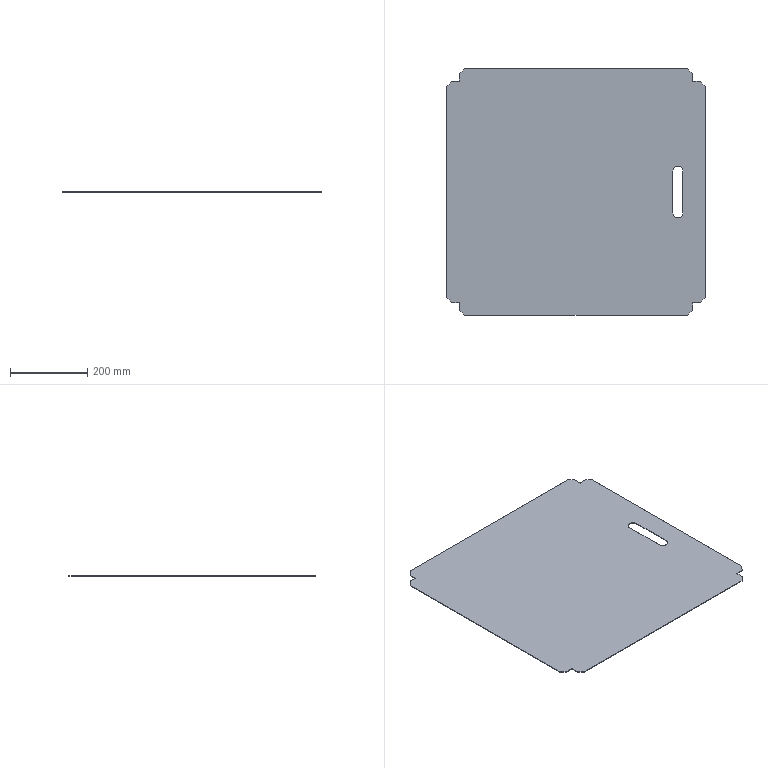Part | SolidWorks | features EdgeFlange 2, FlatPattern 1, ICE 1, SMBaseFlange 1, SheetMetal 1 | 1 solid | 42 faces | box 668.448 x 638.448 x 1.5 mm | volume 627538 mm3 | plane 40 | cylinder 2 | commonest cylinder face diameters 26 x2
STEP:
#1=CARTESIAN_POINT('',(276.5,54.,-1.5));
#2=VERTEX_POINT('',#1);
#3=CARTESIAN_POINT('',(276.5,-54.,-1.5));
#4=VERTEX_POINT('',#3);
#5=CARTESIAN_POINT('',(276.5,54.,-1.5));
#6=DIRECTION('',(0.,-1.,0.));
#7=VECTOR('',#6,1000.);
#8=LINE('',#5,#7);
#9=EDGE_CURVE('',#2,#4,#8,.T.);
#10=ORIENTED_EDGE('',*,*,#9,.F.);
#11=CARTESIAN_POINT('',(250.5,54.,-1.5));
#12=VERTEX_POINT('',#11);
#13=CARTESIAN_POINT('',(263.5,54.,-1.5));
#14=DIRECTION('',(0.,0.,-1.));
#15=DIRECTION('',(-1.,0.,0.));
#16=AXIS2_PLACEMENT_3D('',#13,#14,#15);
#17=CIRCLE('',#16,13.);
#18=EDGE_CURVE('',#12,#2,#17,.T.);
#19=ORIENTED_EDGE('',*,*,#18,.F.);
#20=CARTESIAN_POINT('',(250.5,-54.,-1.5));
#21=VERTEX_POINT('',#20);
#22=CARTESIAN_POINT('',(250.5,54.,-1.5));
#23=DIRECTION('',(0.,1.,0.));
#24=VECTOR('',#23,1000.);
#25=LINE('',#22,#24);
#26=EDGE_CURVE('',#21,#12,#25,.T.);
#27=ORIENTED_EDGE('',*,*,#26,.F.);
#28=CARTESIAN_POINT('',(263.5,-54.,-1.5));
#29=DIRECTION('',(0.,0.,-1.));
#30=DIRECTION('',(-1.,0.,0.));
#31=AXIS2_PLACEMENT_3D('',#28,#29,#30);
#32=CIRCLE('',#31,13.);
#33=EDGE_CURVE('',#4,#21,#32,.T.);
#34=ORIENTED_EDGE('',*,*,#33,.F.);
#35=EDGE_LOOP('',(#10,#19,#27,#34));
#36=FACE_BOUND('',#35,.T.);
#37=CARTESIAN_POINT('',(303.599,-286.293,-1.5));
#38=VERTEX_POINT('',#37);
#39=CARTESIAN_POINT('',(301.263,-286.263,-1.5));
#40=VERTEX_POINT('',#39);
#41=CARTESIAN_POINT('',(303.599,-286.293,-1.5));
#42=DIRECTION('',(-0.9999,0.01263,0.));
#43=VECTOR('',#42,1000.);
#44=LINE('',#41,#43);
#45=EDGE_CURVE('',#38,#40,#44,.T.);
#46=ORIENTED_EDGE('',*,*,#45,.T.);
#47=CARTESIAN_POINT('',(301.293,-286.293,-1.5));
#48=VERTEX_POINT('',#47);
#49=CARTESIAN_POINT('',(301.278,-286.278,-1.5));
#50=DIRECTION('',(-0.7071,0.7071,0.));
#51=VECTOR('',#50,1000.);
#52=LINE('',#49,#51);
#53=EDGE_CURVE('',#48,#40,#52,.T.);
#54=ORIENTED_EDGE('',*,*,#53,.F.);
#55=CARTESIAN_POINT('',(301.293,-304.125,-1.5));
#56=VERTEX_POINT('',#55);
#57=CARTESIAN_POINT('',(301.293,-287.862,-1.5));
#58=DIRECTION('',(0.,-1.,0.));
#59=VECTOR('',#58,1000.);
#60=LINE('',#57,#59);
#61=EDGE_CURVE('',#48,#56,#60,.T.);
#62=ORIENTED_EDGE('',*,*,#61,.T.);
#63=CARTESIAN_POINT('',(300.556,-306.46,-1.5));
#64=VERTEX_POINT('',#63);
#65=CARTESIAN_POINT('',(301.293,-304.125,-1.5));
#66=DIRECTION('',(-0.3008,-0.9537,0.));
#67=VECTOR('',#66,1000.);
#68=LINE('',#65,#67);
#69=EDGE_CURVE('',#56,#64,#68,.T.);
#70=ORIENTED_EDGE('',*,*,#69,.T.);
#71=CARTESIAN_POINT('',(287.793,-319.224,-1.5));
#72=VERTEX_POINT('',#71);
#73=CARTESIAN_POINT('',(-124.592,-731.608,-1.5));
#74=DIRECTION('',(0.7071,0.7071,0.));
#75=VECTOR('',#74,1000.);
#76=LINE('',#73,#75);
#77=EDGE_CURVE('',#72,#64,#76,.T.);
#78=ORIENTED_EDGE('',*,*,#77,.F.);
#79=CARTESIAN_POINT('',(-287.793,-319.224,-1.5));
#80=VERTEX_POINT('',#79);
#81=CARTESIAN_POINT('',(0.,-319.224,-1.5));
#82=DIRECTION('',(-1.,0.,0.));
#83=VECTOR('',#82,1000.);
#84=LINE('',#81,#83);
#85=EDGE_CURVE('',#72,#80,#84,.T.);
#86=ORIENTED_EDGE('',*,*,#85,.T.);
#87=CARTESIAN_POINT('',(-300.556,-306.46,-1.5));
#88=VERTEX_POINT('',#87);
#89=CARTESIAN_POINT('',(-300.556,-306.46,-1.5));
#90=DIRECTION('',(0.7071,-0.7071,0.));
#91=VECTOR('',#90,1000.);
#92=LINE('',#89,#91);
#93=EDGE_CURVE('',#88,#80,#92,.T.);
#94=ORIENTED_EDGE('',*,*,#93,.F.);
#95=CARTESIAN_POINT('',(-301.293,-304.125,-1.5));
#96=VERTEX_POINT('',#95);
#97=CARTESIAN_POINT('',(-300.556,-306.46,-1.5));
#98=DIRECTION('',(-0.3008,0.9537,0.));
#99=VECTOR('',#98,1000.);
#100=LINE('',#97,#99);
#101=EDGE_CURVE('',#88,#96,#100,.T.);
#102=ORIENTED_EDGE('',*,*,#101,.T.);
#103=CARTESIAN_POINT('',(-301.293,-288.599,-1.5));
#104=VERTEX_POINT('',#103);
#105=CARTESIAN_POINT('',(-301.293,-287.862,-1.5));
#106=DIRECTION('',(0.,-1.,0.));
#107=VECTOR('',#106,1000.);
#108=LINE('',#105,#107);
#109=EDGE_CURVE('',#104,#96,#108,.T.);
#110=ORIENTED_EDGE('',*,*,#109,.F.);
#111=CARTESIAN_POINT('',(-301.263,-286.263,-1.5));
#112=VERTEX_POINT('',#111);
#113=CARTESIAN_POINT('',(-301.293,-288.599,-1.5));
#114=DIRECTION('',(0.01263,0.9999,0.));
#115=VECTOR('',#114,1000.);
#116=LINE('',#113,#115);
#117=EDGE_CURVE('',#104,#112,#116,.T.);
#118=ORIENTED_EDGE('',*,*,#117,.T.);
#119=CARTESIAN_POINT('',(-301.293,-286.293,-1.5));
#120=VERTEX_POINT('',#119);
#121=CARTESIAN_POINT('',(-301.278,-286.278,-1.5));
#122=DIRECTION('',(0.7071,0.7071,0.));
#123=VECTOR('',#122,1000.);
#124=LINE('',#121,#123);
#125=EDGE_CURVE('',#120,#112,#124,.T.);
#126=ORIENTED_EDGE('',*,*,#125,.F.);
#127=CARTESIAN_POINT('',(-319.125,-286.293,-1.5));
#128=VERTEX_POINT('',#127);
#129=CARTESIAN_POINT('',(-302.862,-286.293,-1.5));
#130=DIRECTION('',(-1.,0.,0.));
#131=VECTOR('',#130,1000.);
#132=LINE('',#129,#131);
#133=EDGE_CURVE('',#120,#128,#132,.T.);
#134=ORIENTED_EDGE('',*,*,#133,.T.);
#135=CARTESIAN_POINT('',(-321.46,-285.556,-1.5));
#136=VERTEX_POINT('',#135);
#137=CARTESIAN_POINT('',(-319.125,-286.293,-1.5));
#138=DIRECTION('',(-0.9537,0.3008,0.));
#139=VECTOR('',#138,1000.);
#140=LINE('',#137,#139);
#141=EDGE_CURVE('',#128,#136,#140,.T.);
#142=ORIENTED_EDGE('',*,*,#141,.T.);
#143=CARTESIAN_POINT('',(-334.224,-272.793,-1.5));
#144=VERTEX_POINT('',#143);
#145=CARTESIAN_POINT('',(-725.4,118.384,-1.5));
#146=DIRECTION('',(0.7071,-0.7071,0.));
#147=VECTOR('',#146,1000.);
#148=LINE('',#145,#147);
#149=EDGE_CURVE('',#144,#136,#148,.T.);
#150=ORIENTED_EDGE('',*,*,#149,.F.);
#151=CARTESIAN_POINT('',(-334.224,272.793,-1.5));
#152=VERTEX_POINT('',#151);
#153=CARTESIAN_POINT('',(-334.224,0.,-1.5));
#154=DIRECTION('',(0.,1.,0.));
#155=VECTOR('',#154,1000.);
#156=LINE('',#153,#155);
#157=EDGE_CURVE('',#144,#152,#156,.T.);
#158=ORIENTED_EDGE('',*,*,#157,.T.);
#159=CARTESIAN_POINT('',(-321.46,285.556,-1.5));
#160=VERTEX_POINT('',#159);
#161=CARTESIAN_POINT('',(-321.46,285.556,-1.5));
#162=DIRECTION('',(-0.7071,-0.7071,0.));
#163=VECTOR('',#162,1000.);
#164=LINE('',#161,#163);
#165=EDGE_CURVE('',#160,#152,#164,.T.);
#166=ORIENTED_EDGE('',*,*,#165,.F.);
#167=CARTESIAN_POINT('',(-319.125,286.293,-1.5));
#168=VERTEX_POINT('',#167);
#169=CARTESIAN_POINT('',(-321.46,285.556,-1.5));
#170=DIRECTION('',(0.9537,0.3008,0.));
#171=VECTOR('',#170,1000.);
#172=LINE('',#169,#171);
#173=EDGE_CURVE('',#160,#168,#172,.T.);
#174=ORIENTED_EDGE('',*,*,#173,.T.);
#175=CARTESIAN_POINT('',(-303.599,286.293,-1.5));
#176=VERTEX_POINT('',#175);
#177=CARTESIAN_POINT('',(-302.862,286.293,-1.5));
#178=DIRECTION('',(-1.,0.,0.));
#179=VECTOR('',#178,1000.);
#180=LINE('',#177,#179);
#181=EDGE_CURVE('',#176,#168,#180,.T.);
#182=ORIENTED_EDGE('',*,*,#181,.F.);
#183=CARTESIAN_POINT('',(-301.263,286.263,-1.5));
#184=VERTEX_POINT('',#183);
#185=CARTESIAN_POINT('',(-303.599,286.293,-1.5));
#186=DIRECTION('',(0.9999,-0.01263,0.));
#187=VECTOR('',#186,1000.);
#188=LINE('',#185,#187);
#189=EDGE_CURVE('',#176,#184,#188,.T.);
#190=ORIENTED_EDGE('',*,*,#189,.T.);
#191=CARTESIAN_POINT('',(-301.293,286.293,-1.5));
#192=VERTEX_POINT('',#191);
#193=CARTESIAN_POINT('',(-301.278,286.278,-1.5));
#194=DIRECTION('',(0.7071,-0.7071,0.));
#195=VECTOR('',#194,1000.);
#196=LINE('',#193,#195);
#197=EDGE_CURVE('',#192,#184,#196,.T.);
#198=ORIENTED_EDGE('',*,*,#197,.F.);
#199=CARTESIAN_POINT('',(-301.293,304.125,-1.5));
#200=VERTEX_POINT('',#199);
#201=CARTESIAN_POINT('',(-301.293,287.862,-1.5));
#202=DIRECTION('',(0.,1.,0.));
#203=VECTOR('',#202,1000.);
#204=LINE('',#201,#203);
#205=EDGE_CURVE('',#192,#200,#204,.T.);
#206=ORIENTED_EDGE('',*,*,#205,.T.);
#207=CARTESIAN_POINT('',(-300.556,306.46,-1.5));
#208=VERTEX_POINT('',#207);
#209=CARTESIAN_POINT('',(-301.293,304.125,-1.5));
#210=DIRECTION('',(0.3008,0.9537,0.));
#211=VECTOR('',#210,1000.);
#212=LINE('',#209,#211);
#213=EDGE_CURVE('',#200,#208,#212,.T.);
#214=ORIENTED_EDGE('',*,*,#213,.T.);
#215=CARTESIAN_POINT('',(-287.793,319.224,-1.5));
#216=VERTEX_POINT('',#215);
#217=CARTESIAN_POINT('',(124.592,731.608,-1.5));
#218=DIRECTION('',(-0.7071,-0.7071,0.));
#219=VECTOR('',#218,1000.);
#220=LINE('',#217,#219);
#221=EDGE_CURVE('',#216,#208,#220,.T.);
#222=ORIENTED_EDGE('',*,*,#221,.F.);
#223=CARTESIAN_POINT('',(287.793,319.224,-1.5));
#224=VERTEX_POINT('',#223);
#225=CARTESIAN_POINT('',(0.,319.224,-1.5));
#226=DIRECTION('',(1.,0.,0.));
#227=VECTOR('',#226,1000.);
#228=LINE('',#225,#227);
#229=EDGE_CURVE('',#216,#224,#228,.T.);
#230=ORIENTED_EDGE('',*,*,#229,.T.);
#231=CARTESIAN_POINT('',(300.556,306.46,-1.5));
#232=VERTEX_POINT('',#231);
#233=CARTESIAN_POINT('',(300.556,306.46,-1.5));
#234=DIRECTION('',(-0.7071,0.7071,0.));
#235=VECTOR('',#234,1000.);
#236=LINE('',#233,#235);
#237=EDGE_CURVE('',#232,#224,#236,.T.);
#238=ORIENTED_EDGE('',*,*,#237,.F.);
#239=CARTESIAN_POINT('',(301.293,304.125,-1.5));
#240=VERTEX_POINT('',#239);
#241=CARTESIAN_POINT('',(300.556,306.46,-1.5));
#242=DIRECTION('',(0.3008,-0.9537,0.));
#243=VECTOR('',#242,1000.);
#244=LINE('',#241,#243);
#245=EDGE_CURVE('',#232,#240,#244,.T.);
#246=ORIENTED_EDGE('',*,*,#245,.T.);
#247=CARTESIAN_POINT('',(301.293,288.599,-1.5));
#248=VERTEX_POINT('',#247);
#249=CARTESIAN_POINT('',(301.293,287.862,-1.5));
#250=DIRECTION('',(0.,1.,0.));
#251=VECTOR('',#250,1000.);
#252=LINE('',#249,#251);
#253=EDGE_CURVE('',#248,#240,#252,.T.);
#254=ORIENTED_EDGE('',*,*,#253,.F.);
#255=CARTESIAN_POINT('',(301.263,286.263,-1.5));
#256=VERTEX_POINT('',#255);
#257=CARTESIAN_POINT('',(301.293,288.599,-1.5));
#258=DIRECTION('',(-0.01263,-0.9999,0.));
#259=VECTOR('',#258,1000.);
#260=LINE('',#257,#259);
#261=EDGE_CURVE('',#248,#256,#260,.T.);
#262=ORIENTED_EDGE('',*,*,#261,.T.);
#263=CARTESIAN_POINT('',(301.293,286.293,-1.5));
#264=VERTEX_POINT('',#263);
#265=CARTESIAN_POINT('',(301.278,286.278,-1.5));
#266=DIRECTION('',(-0.7071,-0.7071,0.));
#267=VECTOR('',#266,1000.);
#268=LINE('',#265,#267);
#269=EDGE_CURVE('',#264,#256,#268,.T.);
#270=ORIENTED_EDGE('',*,*,#269,.F.);
#271=CARTESIAN_POINT('',(319.125,286.293,-1.5));
#272=VERTEX_POINT('',#271);
#273=CARTESIAN_POINT('',(302.862,286.293,-1.5));
#274=DIRECTION('',(1.,0.,0.));
#275=VECTOR('',#274,1000.);
#276=LINE('',#273,#275);
#277=EDGE_CURVE('',#264,#272,#276,.T.);
#278=ORIENTED_EDGE('',*,*,#277,.T.);
#279=CARTESIAN_POINT('',(321.46,285.556,-1.5));
#280=VERTEX_POINT('',#279);
#281=CARTESIAN_POINT('',(319.125,286.293,-1.5));
#282=DIRECTION('',(0.9537,-0.3008,0.));
#283=VECTOR('',#282,1000.);
#284=LINE('',#281,#283);
#285=EDGE_CURVE('',#272,#280,#284,.T.);
#286=ORIENTED_EDGE('',*,*,#285,.T.);
#287=CARTESIAN_POINT('',(334.224,272.793,-1.5));
#288=VERTEX_POINT('',#287);
#289=CARTESIAN_POINT('',(725.4,-118.384,-1.5));
#290=DIRECTION('',(-0.7071,0.7071,0.));
#291=VECTOR('',#290,1000.);
#292=LINE('',#289,#291);
#293=EDGE_CURVE('',#288,#280,#292,.T.);
#294=ORIENTED_EDGE('',*,*,#293,.F.);
#295=CARTESIAN_POINT('',(334.224,-272.793,-1.5));
#296=VERTEX_POINT('',#295);
#297=CARTESIAN_POINT('',(334.224,0.,-1.5));
#298=DIRECTION('',(0.,-1.,0.));
#299=VECTOR('',#298,1000.);
#300=LINE('',#297,#299);
#301=EDGE_CURVE('',#288,#296,#300,.T.);
#302=ORIENTED_EDGE('',*,*,#301,.T.);
#303=CARTESIAN_POINT('',(321.46,-285.556,-1.5));
#304=VERTEX_POINT('',#303);
#305=CARTESIAN_POINT('',(321.46,-285.556,-1.5));
#306=DIRECTION('',(0.7071,0.7071,0.));
#307=VECTOR('',#306,1000.);
#308=LINE('',#305,#307);
#309=EDGE_CURVE('',#304,#296,#308,.T.);
#310=ORIENTED_EDGE('',*,*,#309,.F.);
#311=CARTESIAN_POINT('',(319.125,-286.293,-1.5));
#312=VERTEX_POINT('',#311);
#313=CARTESIAN_POINT('',(321.46,-285.556,-1.5));
#314=DIRECTION('',(-0.9537,-0.3008,0.));
#315=VECTOR('',#314,1000.);
#316=LINE('',#313,#315);
#317=EDGE_CURVE('',#304,#312,#316,.T.);
#318=ORIENTED_EDGE('',*,*,#317,.T.);
#319=CARTESIAN_POINT('',(302.862,-286.293,-1.5));
#320=DIRECTION('',(1.,0.,0.));
#321=VECTOR('',#320,1000.);
#322=LINE('',#319,#321);
#323=EDGE_CURVE('',#38,#312,#322,.T.);
#324=ORIENTED_EDGE('',*,*,#323,.F.);
#325=EDGE_LOOP('',(#46,#54,#62,#70,#78,#86,#94,#102,#110,#118,#126,#134,#142,#150,#158,#166,#174,#182,#190,#198,#206,#214,#222,#230,#238,#246,#254,#262,#270,#278,#286,#294,#302,#310,#318,#324));
#326=FACE_OUTER_BOUND('',#325,.T.);
#327=CARTESIAN_POINT('',(0.,0.,-1.5));
#328=DIRECTION('',(0.,0.,1.));
#329=DIRECTION('',(1.,0.,0.));
#330=AXIS2_PLACEMENT_3D('',#327,#328,#329);
#331=PLANE('',#330);
#332=ADVANCED_FACE('',(#36,#326),#331,.F.);
#333=CARTESIAN_POINT('',(276.5,54.,0.));
#334=VERTEX_POINT('',#333);
#335=CARTESIAN_POINT('',(250.5,54.,0.));
#336=VERTEX_POINT('',#335);
#337=CARTESIAN_POINT('',(263.5,54.,0.));
#338=DIRECTION('',(0.,0.,1.));
#339=DIRECTION('',(1.,0.,0.));
#340=AXIS2_PLACEMENT_3D('',#337,#338,#339);
#341=CIRCLE('',#340,13.);
#342=EDGE_CURVE('',#334,#336,#341,.T.);
#343=ORIENTED_EDGE('',*,*,#342,.F.);
#344=CARTESIAN_POINT('',(276.5,-54.,0.));
#345=VERTEX_POINT('',#344);
#346=CARTESIAN_POINT('',(276.5,0.,0.));
#347=DIRECTION('',(0.,1.,0.));
#348=VECTOR('',#347,1000.);
#349=LINE('',#346,#348);
#350=EDGE_CURVE('',#345,#334,#349,.T.);
#351=ORIENTED_EDGE('',*,*,#350,.F.);
#352=CARTESIAN_POINT('',(250.5,-54.,0.));
#353=VERTEX_POINT('',#352);
#354=CARTESIAN_POINT('',(263.5,-54.,0.));
#355=DIRECTION('',(0.,0.,1.));
#356=DIRECTION('',(1.,0.,0.));
#357=AXIS2_PLACEMENT_3D('',#354,#355,#356);
#358=CIRCLE('',#357,13.);
#359=EDGE_CURVE('',#353,#345,#358,.T.);
#360=ORIENTED_EDGE('',*,*,#359,.F.);
#361=CARTESIAN_POINT('',(250.5,0.,0.));
#362=DIRECTION('',(0.,-1.,0.));
#363=VECTOR('',#362,1000.);
#364=LINE('',#361,#363);
#365=EDGE_CURVE('',#336,#353,#364,.T.);
#366=ORIENTED_EDGE('',*,*,#365,.F.);
#367=EDGE_LOOP('',(#343,#351,#360,#366));
#368=FACE_BOUND('',#367,.T.);
#369=CARTESIAN_POINT('',(-301.293,-286.293,0.));
#370=VERTEX_POINT('',#369);
#371=CARTESIAN_POINT('',(-301.263,-286.263,0.));
#372=VERTEX_POINT('',#371);
#373=CARTESIAN_POINT('',(-301.278,-286.278,0.));
#374=DIRECTION('',(0.7071,0.7071,0.));
#375=VECTOR('',#374,1000.);
#376=LINE('',#373,#375);
#377=EDGE_CURVE('',#370,#372,#376,.T.);
#378=ORIENTED_EDGE('',*,*,#377,.T.);
#379=CARTESIAN_POINT('',(-301.293,-288.599,0.));
#380=VERTEX_POINT('',#379);
#381=CARTESIAN_POINT('',(-301.293,-288.599,0.));
#382=DIRECTION('',(0.01263,0.9999,0.));
#383=VECTOR('',#382,1000.);
#384=LINE('',#381,#383);
#385=EDGE_CURVE('',#380,#372,#384,.T.);
#386=ORIENTED_EDGE('',*,*,#385,.F.);
#387=CARTESIAN_POINT('',(-301.293,-304.125,0.));
#388=VERTEX_POINT('',#387);
#389=CARTESIAN_POINT('',(-301.293,-287.862,0.));
#390=DIRECTION('',(0.,-1.,0.));
#391=VECTOR('',#390,1000.);
#392=LINE('',#389,#391);
#393=EDGE_CURVE('',#380,#388,#392,.T.);
#394=ORIENTED_EDGE('',*,*,#393,.T.);
#395=CARTESIAN_POINT('',(-300.556,-306.46,0.));
#396=VERTEX_POINT('',#395);
#397=CARTESIAN_POINT('',(-300.556,-306.46,0.));
#398=DIRECTION('',(-0.3008,0.9537,0.));
#399=VECTOR('',#398,1000.);
#400=LINE('',#397,#399);
#401=EDGE_CURVE('',#396,#388,#400,.T.);
#402=ORIENTED_EDGE('',*,*,#401,.F.);
#403=CARTESIAN_POINT('',(-287.793,-319.224,0.));
#404=VERTEX_POINT('',#403);
#405=CARTESIAN_POINT('',(-7.146,-599.87,0.));
#406=DIRECTION('',(0.7071,-0.7071,0.));
#407=VECTOR('',#406,1000.);
#408=LINE('',#405,#407);
#409=EDGE_CURVE('',#396,#404,#408,.T.);
#410=ORIENTED_EDGE('',*,*,#409,.T.);
#411=CARTESIAN_POINT('',(287.793,-319.224,0.));
#412=VERTEX_POINT('',#411);
#413=CARTESIAN_POINT('',(-301.293,-319.224,0.));
#414=DIRECTION('',(-1.,0.,0.));
#415=VECTOR('',#414,1000.);
#416=LINE('',#413,#415);
#417=EDGE_CURVE('',#412,#404,#416,.T.);
#418=ORIENTED_EDGE('',*,*,#417,.F.);
#419=CARTESIAN_POINT('',(300.556,-306.46,0.));
#420=VERTEX_POINT('',#419);
#421=CARTESIAN_POINT('',(7.146,-599.87,0.));
#422=DIRECTION('',(0.7071,0.7071,0.));
#423=VECTOR('',#422,1000.);
#424=LINE('',#421,#423);
#425=EDGE_CURVE('',#412,#420,#424,.T.);
#426=ORIENTED_EDGE('',*,*,#425,.T.);
#427=CARTESIAN_POINT('',(301.293,-304.125,0.));
#428=VERTEX_POINT('',#427);
#429=CARTESIAN_POINT('',(301.293,-304.125,0.));
#430=DIRECTION('',(-0.3008,-0.9537,0.));
#431=VECTOR('',#430,1000.);
#432=LINE('',#429,#431);
#433=EDGE_CURVE('',#428,#420,#432,.T.);
#434=ORIENTED_EDGE('',*,*,#433,.F.);
#435=CARTESIAN_POINT('',(301.293,-286.293,0.));
#436=VERTEX_POINT('',#435);
#437=CARTESIAN_POINT('',(301.293,-287.862,0.));
#438=DIRECTION('',(0.,-1.,0.));
#439=VECTOR('',#438,1000.);
#440=LINE('',#437,#439);
#441=EDGE_CURVE('',#436,#428,#440,.T.);
#442=ORIENTED_EDGE('',*,*,#441,.F.);
#443=CARTESIAN_POINT('',(301.263,-286.263,0.));
#444=VERTEX_POINT('',#443);
#445=CARTESIAN_POINT('',(301.278,-286.278,0.));
#446=DIRECTION('',(-0.7071,0.7071,0.));
#447=VECTOR('',#446,1000.);
#448=LINE('',#445,#447);
#449=EDGE_CURVE('',#436,#444,#448,.T.);
#450=ORIENTED_EDGE('',*,*,#449,.T.);
#451=CARTESIAN_POINT('',(303.599,-286.293,0.));
#452=VERTEX_POINT('',#451);
#453=CARTESIAN_POINT('',(303.599,-286.293,0.));
#454=DIRECTION('',(-0.9999,0.01263,0.));
#455=VECTOR('',#454,1000.);
#456=LINE('',#453,#455);
#457=EDGE_CURVE('',#452,#444,#456,.T.);
#458=ORIENTED_EDGE('',*,*,#457,.F.);
#459=CARTESIAN_POINT('',(319.125,-286.293,0.));
#460=VERTEX_POINT('',#459);
#461=CARTESIAN_POINT('',(302.862,-286.293,0.));
#462=DIRECTION('',(1.,0.,0.));
#463=VECTOR('',#462,1000.);
#464=LINE('',#461,#463);
#465=EDGE_CURVE('',#452,#460,#464,.T.);
#466=ORIENTED_EDGE('',*,*,#465,.T.);
#467=CARTESIAN_POINT('',(321.46,-285.556,0.));
#468=VERTEX_POINT('',#467);
#469=CARTESIAN_POINT('',(321.46,-285.556,0.));
#470=DIRECTION('',(-0.9537,-0.3008,0.));
#471=VECTOR('',#470,1000.);
#472=LINE('',#469,#471);
#473=EDGE_CURVE('',#468,#460,#472,.T.);
#474=ORIENTED_EDGE('',*,*,#473,.F.);
#475=CARTESIAN_POINT('',(334.224,-272.793,0.));
#476=VERTEX_POINT('',#475);
#477=CARTESIAN_POINT('',(614.87,7.854,0.));
#478=DIRECTION('',(0.7071,0.7071,0.));
#479=VECTOR('',#478,1000.);
#480=LINE('',#477,#479);
#481=EDGE_CURVE('',#468,#476,#480,.T.);
#482=ORIENTED_EDGE('',*,*,#481,.T.);
#483=CARTESIAN_POINT('',(334.224,272.793,0.));
#484=VERTEX_POINT('',#483);
#485=CARTESIAN_POINT('',(334.224,-286.293,0.));
#486=DIRECTION('',(0.,-1.,0.));
#487=VECTOR('',#486,1000.);
#488=LINE('',#485,#487);
#489=EDGE_CURVE('',#484,#476,#488,.T.);
#490=ORIENTED_EDGE('',*,*,#489,.F.);
#491=CARTESIAN_POINT('',(321.46,285.556,0.));
#492=VERTEX_POINT('',#491);
#493=CARTESIAN_POINT('',(614.87,-7.854,0.));
#494=DIRECTION('',(-0.7071,0.7071,0.));
#495=VECTOR('',#494,1000.);
#496=LINE('',#493,#495);
#497=EDGE_CURVE('',#484,#492,#496,.T.);
#498=ORIENTED_EDGE('',*,*,#497,.T.);
#499=CARTESIAN_POINT('',(319.125,286.293,0.));
#500=VERTEX_POINT('',#499);
#501=CARTESIAN_POINT('',(319.125,286.293,0.));
#502=DIRECTION('',(0.9537,-0.3008,0.));
#503=VECTOR('',#502,1000.);
#504=LINE('',#501,#503);
#505=EDGE_CURVE('',#500,#492,#504,.T.);
#506=ORIENTED_EDGE('',*,*,#505,.F.);
#507=CARTESIAN_POINT('',(301.293,286.293,0.));
#508=VERTEX_POINT('',#507);
#509=CARTESIAN_POINT('',(302.862,286.293,0.));
#510=DIRECTION('',(1.,0.,0.));
#511=VECTOR('',#510,1000.);
#512=LINE('',#509,#511);
#513=EDGE_CURVE('',#508,#500,#512,.T.);
#514=ORIENTED_EDGE('',*,*,#513,.F.);
#515=CARTESIAN_POINT('',(301.263,286.263,0.));
#516=VERTEX_POINT('',#515);
#517=CARTESIAN_POINT('',(301.278,286.278,0.));
#518=DIRECTION('',(-0.7071,-0.7071,0.));
#519=VECTOR('',#518,1000.);
#520=LINE('',#517,#519);
#521=EDGE_CURVE('',#508,#516,#520,.T.);
#522=ORIENTED_EDGE('',*,*,#521,.T.);
#523=CARTESIAN_POINT('',(301.293,288.599,0.));
#524=VERTEX_POINT('',#523);
#525=CARTESIAN_POINT('',(301.293,288.599,0.));
#526=DIRECTION('',(-0.01263,-0.9999,0.));
#527=VECTOR('',#526,1000.);
#528=LINE('',#525,#527);
#529=EDGE_CURVE('',#524,#516,#528,.T.);
#530=ORIENTED_EDGE('',*,*,#529,.F.);
#531=CARTESIAN_POINT('',(301.293,304.125,0.));
#532=VERTEX_POINT('',#531);
#533=CARTESIAN_POINT('',(301.293,287.862,0.));
#534=DIRECTION('',(0.,1.,0.));
#535=VECTOR('',#534,1000.);
#536=LINE('',#533,#535);
#537=EDGE_CURVE('',#524,#532,#536,.T.);
#538=ORIENTED_EDGE('',*,*,#537,.T.);
#539=CARTESIAN_POINT('',(300.556,306.46,0.));
#540=VERTEX_POINT('',#539);
#541=CARTESIAN_POINT('',(300.556,306.46,0.));
#542=DIRECTION('',(0.3008,-0.9537,0.));
#543=VECTOR('',#542,1000.);
#544=LINE('',#541,#543);
#545=EDGE_CURVE('',#540,#532,#544,.T.);
#546=ORIENTED_EDGE('',*,*,#545,.F.);
#547=CARTESIAN_POINT('',(287.793,319.224,0.));
#548=VERTEX_POINT('',#547);
#549=CARTESIAN_POINT('',(7.146,599.87,0.));
#550=DIRECTION('',(-0.7071,0.7071,0.));
#551=VECTOR('',#550,1000.);
#552=LINE('',#549,#551);
#553=EDGE_CURVE('',#540,#548,#552,.T.);
#554=ORIENTED_EDGE('',*,*,#553,.T.);
#555=CARTESIAN_POINT('',(-287.793,319.224,0.));
#556=VERTEX_POINT('',#555);
#557=CARTESIAN_POINT('',(301.293,319.224,0.));
#558=DIRECTION('',(1.,0.,0.));
#559=VECTOR('',#558,1000.);
#560=LINE('',#557,#559);
#561=EDGE_CURVE('',#556,#548,#560,.T.);
#562=ORIENTED_EDGE('',*,*,#561,.F.);
#563=CARTESIAN_POINT('',(-300.556,306.46,0.));
#564=VERTEX_POINT('',#563);
#565=CARTESIAN_POINT('',(-7.146,599.87,0.));
#566=DIRECTION('',(-0.7071,-0.7071,0.));
#567=VECTOR('',#566,1000.);
#568=LINE('',#565,#567);
#569=EDGE_CURVE('',#556,#564,#568,.T.);
#570=ORIENTED_EDGE('',*,*,#569,.T.);
#571=CARTESIAN_POINT('',(-301.293,304.125,0.));
#572=VERTEX_POINT('',#571);
#573=CARTESIAN_POINT('',(-301.293,304.125,0.));
#574=DIRECTION('',(0.3008,0.9537,0.));
#575=VECTOR('',#574,1000.);
#576=LINE('',#573,#575);
#577=EDGE_CURVE('',#572,#564,#576,.T.);
#578=ORIENTED_EDGE('',*,*,#577,.F.);
#579=CARTESIAN_POINT('',(-301.293,286.293,0.));
#580=VERTEX_POINT('',#579);
#581=CARTESIAN_POINT('',(-301.293,287.862,0.));
#582=DIRECTION('',(0.,1.,0.));
#583=VECTOR('',#582,1000.);
#584=LINE('',#581,#583);
#585=EDGE_CURVE('',#580,#572,#584,.T.);
#586=ORIENTED_EDGE('',*,*,#585,.F.);
#587=CARTESIAN_POINT('',(-301.263,286.263,0.));
#588=VERTEX_POINT('',#587);
#589=CARTESIAN_POINT('',(-301.278,286.278,0.));
#590=DIRECTION('',(0.7071,-0.7071,0.));
#591=VECTOR('',#590,1000.);
#592=LINE('',#589,#591);
#593=EDGE_CURVE('',#580,#588,#592,.T.);
#594=ORIENTED_EDGE('',*,*,#593,.T.);
#595=CARTESIAN_POINT('',(-303.599,286.293,0.));
#596=VERTEX_POINT('',#595);
#597=CARTESIAN_POINT('',(-303.599,286.293,0.));
#598=DIRECTION('',(0.9999,-0.01263,0.));
#599=VECTOR('',#598,1000.);
#600=LINE('',#597,#599);
#601=EDGE_CURVE('',#596,#588,#600,.T.);
#602=ORIENTED_EDGE('',*,*,#601,.F.);
#603=CARTESIAN_POINT('',(-319.125,286.293,0.));
#604=VERTEX_POINT('',#603);
#605=CARTESIAN_POINT('',(-302.862,286.293,0.));
#606=DIRECTION('',(-1.,0.,0.));
#607=VECTOR('',#606,1000.);
#608=LINE('',#605,#607);
#609=EDGE_CURVE('',#596,#604,#608,.T.);
#610=ORIENTED_EDGE('',*,*,#609,.T.);
#611=CARTESIAN_POINT('',(-321.46,285.556,0.));
#612=VERTEX_POINT('',#611);
#613=CARTESIAN_POINT('',(-321.46,285.556,0.));
#614=DIRECTION('',(0.9537,0.3008,0.));
#615=VECTOR('',#614,1000.);
#616=LINE('',#613,#615);
#617=EDGE_CURVE('',#612,#604,#616,.T.);
#618=ORIENTED_EDGE('',*,*,#617,.F.);
#619=CARTESIAN_POINT('',(-334.224,272.793,0.));
#620=VERTEX_POINT('',#619);
#621=CARTESIAN_POINT('',(-614.87,-7.854,0.));
#622=DIRECTION('',(-0.7071,-0.7071,0.));
#623=VECTOR('',#622,1000.);
#624=LINE('',#621,#623);
#625=EDGE_CURVE('',#612,#620,#624,.T.);
#626=ORIENTED_EDGE('',*,*,#625,.T.);
#627=CARTESIAN_POINT('',(-334.224,-272.793,0.));
#628=VERTEX_POINT('',#627);
#629=CARTESIAN_POINT('',(-334.224,286.293,0.));
#630=DIRECTION('',(0.,1.,0.));
#631=VECTOR('',#630,1000.);
#632=LINE('',#629,#631);
#633=EDGE_CURVE('',#628,#620,#632,.T.);
#634=ORIENTED_EDGE('',*,*,#633,.F.);
#635=CARTESIAN_POINT('',(-321.46,-285.556,0.));
#636=VERTEX_POINT('',#635);
#637=CARTESIAN_POINT('',(-614.87,7.854,0.));
#638=DIRECTION('',(0.7071,-0.7071,0.));
#639=VECTOR('',#638,1000.);
#640=LINE('',#637,#639);
#641=EDGE_CURVE('',#628,#636,#640,.T.);
#642=ORIENTED_EDGE('',*,*,#641,.T.);
#643=CARTESIAN_POINT('',(-319.125,-286.293,0.));
#644=VERTEX_POINT('',#643);
#645=CARTESIAN_POINT('',(-319.125,-286.293,0.));
#646=DIRECTION('',(-0.9537,0.3008,0.));
#647=VECTOR('',#646,1000.);
#648=LINE('',#645,#647);
#649=EDGE_CURVE('',#644,#636,#648,.T.);
#650=ORIENTED_EDGE('',*,*,#649,.F.);
#651=CARTESIAN_POINT('',(-302.862,-286.293,0.));
#652=DIRECTION('',(-1.,0.,0.));
#653=VECTOR('',#652,1000.);
#654=LINE('',#651,#653);
#655=EDGE_CURVE('',#370,#644,#654,.T.);
#656=ORIENTED_EDGE('',*,*,#655,.F.);
#657=EDGE_LOOP('',(#378,#386,#394,#402,#410,#418,#426,#434,#442,#450,#458,#466,#474,#482,#490,#498,#506,#514,#522,#530,#538,#546,#554,#562,#570,#578,#586,#594,#602,#610,#618,#626,#634,#642,#650,#656));
#658=FACE_OUTER_BOUND('',#657,.T.);
#659=CARTESIAN_POINT('',(0.,0.,0.));
#660=DIRECTION('',(0.,0.,1.));
#661=DIRECTION('',(1.,0.,0.));
#662=AXIS2_PLACEMENT_3D('',#659,#660,#661);
#663=PLANE('',#662);
#664=ADVANCED_FACE('',(#368,#658),#663,.T.);
#665=ORIENTED_EDGE('',*,*,#342,.T.);
#666=CARTESIAN_POINT('',(250.5,54.,8.5));
#667=DIRECTION('',(0.,0.,-1.));
#668=VECTOR('',#667,1000.);
#669=LINE('',#666,#668);
#670=EDGE_CURVE('',#336,#12,#669,.T.);
#671=ORIENTED_EDGE('',*,*,#670,.T.);
#672=ORIENTED_EDGE('',*,*,#18,.T.);
#673=CARTESIAN_POINT('',(276.5,54.,8.5));
#674=DIRECTION('',(0.,0.,-1.));
#675=VECTOR('',#674,1000.);
#676=LINE('',#673,#675);
#677=EDGE_CURVE('',#334,#2,#676,.T.);
#678=ORIENTED_EDGE('',*,*,#677,.F.);
#679=EDGE_LOOP('',(#665,#671,#672,#678));
#680=FACE_OUTER_BOUND('',#679,.T.);
#681=CARTESIAN_POINT('',(263.5,54.,8.5));
#682=DIRECTION('',(0.,0.,-1.));
#683=DIRECTION('',(-1.,0.,0.));
#684=AXIS2_PLACEMENT_3D('',#681,#682,#683);
#685=CYLINDRICAL_SURFACE('',#684,13.);
#686=ADVANCED_FACE('',(#680),#685,.F.);
#687=ORIENTED_EDGE('',*,*,#365,.T.);
#688=CARTESIAN_POINT('',(250.5,-54.,8.5));
#689=DIRECTION('',(0.,0.,-1.));
#690=VECTOR('',#689,1000.);
#691=LINE('',#688,#690);
#692=EDGE_CURVE('',#353,#21,#691,.T.);
#693=ORIENTED_EDGE('',*,*,#692,.T.);
#694=ORIENTED_EDGE('',*,*,#26,.T.);
#695=ORIENTED_EDGE('',*,*,#670,.F.);
#696=EDGE_LOOP('',(#687,#693,#694,#695));
#697=FACE_OUTER_BOUND('',#696,.T.);
#698=CARTESIAN_POINT('',(250.5,54.,8.5));
#699=DIRECTION('',(-1.,0.,0.));
#700=DIRECTION('',(0.,-1.,0.));
#701=AXIS2_PLACEMENT_3D('',#698,#699,#700);
#702=PLANE('',#701);
#703=ADVANCED_FACE('',(#697),#702,.F.);
#704=ORIENTED_EDGE('',*,*,#359,.T.);
#705=CARTESIAN_POINT('',(276.5,-54.,8.5));
#706=DIRECTION('',(0.,0.,-1.));
#707=VECTOR('',#706,1000.);
#708=LINE('',#705,#707);
#709=EDGE_CURVE('',#345,#4,#708,.T.);
#710=ORIENTED_EDGE('',*,*,#709,.T.);
#711=ORIENTED_EDGE('',*,*,#33,.T.);
#712=ORIENTED_EDGE('',*,*,#692,.F.);
#713=EDGE_LOOP('',(#704,#710,#711,#712));
#714=FACE_OUTER_BOUND('',#713,.T.);
#715=CARTESIAN_POINT('',(263.5,-54.,8.5));
#716=DIRECTION('',(0.,0.,-1.));
#717=DIRECTION('',(-1.,0.,0.));
#718=AXIS2_PLACEMENT_3D('',#715,#716,#717);
#719=CYLINDRICAL_SURFACE('',#718,13.);
#720=ADVANCED_FACE('',(#714),#719,.F.);
#721=ORIENTED_EDGE('',*,*,#350,.T.);
#722=ORIENTED_EDGE('',*,*,#677,.T.);
#723=ORIENTED_EDGE('',*,*,#9,.T.);
#724=ORIENTED_EDGE('',*,*,#709,.F.);
#725=EDGE_LOOP('',(#721,#722,#723,#724));
#726=FACE_OUTER_BOUND('',#725,.T.);
#727=CARTESIAN_POINT('',(276.5,54.,8.5));
#728=DIRECTION('',(1.,0.,0.));
#729=DIRECTION('',(0.,0.,-1.));
#730=AXIS2_PLACEMENT_3D('',#727,#728,#729);
#731=PLANE('',#730);
#732=ADVANCED_FACE('',(#726),#731,.F.);
#733=ORIENTED_EDGE('',*,*,#385,.T.);
#734=CARTESIAN_POINT('',(-301.263,-286.263,0.));
#735=DIRECTION('',(0.,0.,-1.));
#736=VECTOR('',#735,1000.);
#737=LINE('',#734,#736);
#738=EDGE_CURVE('',#372,#112,#737,.T.);
#739=ORIENTED_EDGE('',*,*,#738,.T.);
#740=ORIENTED_EDGE('',*,*,#117,.F.);
#741=CARTESIAN_POINT('',(-301.293,-288.599,0.));
#742=DIRECTION('',(0.,0.,1.));
#743=VECTOR('',#742,1000.);
#744=LINE('',#741,#743);
#745=EDGE_CURVE('',#104,#380,#744,.T.);
#746=ORIENTED_EDGE('',*,*,#745,.T.);
#747=EDGE_LOOP('',(#733,#739,#740,#746));
#748=FACE_OUTER_BOUND('',#747,.T.);
#749=CARTESIAN_POINT('',(-301.293,-288.599,-0.75));
#750=DIRECTION('',(-0.9999,0.01263,0.));
#751=DIRECTION('',(0.01263,0.9999,0.));
#752=AXIS2_PLACEMENT_3D('',#749,#750,#751);
#753=PLANE('',#752);
#754=ADVANCED_FACE('',(#748),#753,.T.);
#755=CARTESIAN_POINT('',(-287.793,-319.224,-1.5));
#756=DIRECTION('',(0.,0.,1.));
#757=VECTOR('',#756,1000.);
#758=LINE('',#755,#757);
#759=EDGE_CURVE('',#80,#404,#758,.T.);
#760=ORIENTED_EDGE('',*,*,#759,.F.);
#761=ORIENTED_EDGE('',*,*,#85,.F.);
#762=CARTESIAN_POINT('',(287.793,-319.224,-1.5));
#763=DIRECTION('',(0.,0.,-1.));
#764=VECTOR('',#763,1000.);
#765=LINE('',#762,#764);
#766=EDGE_CURVE('',#412,#72,#765,.T.);
#767=ORIENTED_EDGE('',*,*,#766,.F.);
#768=ORIENTED_EDGE('',*,*,#417,.T.);
#769=EDGE_LOOP('',(#760,#761,#767,#768));
#770=FACE_OUTER_BOUND('',#769,.T.);
#771=CARTESIAN_POINT('',(-301.293,-319.224,-1.5));
#772=DIRECTION('',(0.,1.,0.));
#773=DIRECTION('',(0.,0.,1.));
#774=AXIS2_PLACEMENT_3D('',#771,#772,#773);
#775=PLANE('',#774);
#776=ADVANCED_FACE('',(#770),#775,.F.);
#777=ORIENTED_EDGE('',*,*,#409,.F.);
#778=CARTESIAN_POINT('',(-300.556,-306.46,0.));
#779=DIRECTION('',(0.,0.,1.));
#780=VECTOR('',#779,1000.);
#781=LINE('',#778,#780);
#782=EDGE_CURVE('',#88,#396,#781,.T.);
#783=ORIENTED_EDGE('',*,*,#782,.F.);
#784=ORIENTED_EDGE('',*,*,#93,.T.);
#785=ORIENTED_EDGE('',*,*,#759,.T.);
#786=EDGE_LOOP('',(#777,#783,#784,#785));
#787=FACE_OUTER_BOUND('',#786,.T.);
#788=CARTESIAN_POINT('',(-300.556,-306.46,-1.5));
#789=DIRECTION('',(-0.7071,-0.7071,0.));
#790=DIRECTION('',(-0.7071,0.7071,0.));
#791=AXIS2_PLACEMENT_3D('',#788,#789,#790);
#792=PLANE('',#791);
#793=ADVANCED_FACE('',(#787),#792,.T.);
#794=ORIENTED_EDGE('',*,*,#425,.F.);
#795=ORIENTED_EDGE('',*,*,#766,.T.);
#796=ORIENTED_EDGE('',*,*,#77,.T.);
#797=CARTESIAN_POINT('',(300.556,-306.46,0.));
#798=DIRECTION('',(0.,0.,1.));
#799=VECTOR('',#798,1000.);
#800=LINE('',#797,#799);
#801=EDGE_CURVE('',#64,#420,#800,.T.);
#802=ORIENTED_EDGE('',*,*,#801,.T.);
#803=EDGE_LOOP('',(#794,#795,#796,#802));
#804=FACE_OUTER_BOUND('',#803,.T.);
#805=CARTESIAN_POINT('',(-124.592,-731.608,-1.5));
#806=DIRECTION('',(0.7071,-0.7071,0.));
#807=DIRECTION('',(-0.7071,-0.7071,0.));
#808=AXIS2_PLACEMENT_3D('',#805,#806,#807);
#809=PLANE('',#808);
#810=ADVANCED_FACE('',(#804),#809,.T.);
#811=ORIENTED_EDGE('',*,*,#401,.T.);
#812=CARTESIAN_POINT('',(-301.293,-304.125,0.));
#813=DIRECTION('',(0.,0.,-1.));
#814=VECTOR('',#813,1000.);
#815=LINE('',#812,#814);
#816=EDGE_CURVE('',#388,#96,#815,.T.);
#817=ORIENTED_EDGE('',*,*,#816,.T.);
#818=ORIENTED_EDGE('',*,*,#101,.F.);
#819=ORIENTED_EDGE('',*,*,#782,.T.);
#820=EDGE_LOOP('',(#811,#817,#818,#819));
#821=FACE_OUTER_BOUND('',#820,.T.);
#822=CARTESIAN_POINT('',(-300.556,-306.46,-0.75));
#823=DIRECTION('',(-0.9537,-0.3008,0.));
#824=DIRECTION('',(-0.3008,0.9537,0.));
#825=AXIS2_PLACEMENT_3D('',#822,#823,#824);
#826=PLANE('',#825);
#827=ADVANCED_FACE('',(#821),#826,.T.);
#828=CARTESIAN_POINT('',(301.293,-304.125,0.));
#829=DIRECTION('',(0.,0.,-1.));
#830=VECTOR('',#829,1000.);
#831=LINE('',#828,#830);
#832=EDGE_CURVE('',#428,#56,#831,.T.);
#833=ORIENTED_EDGE('',*,*,#832,.F.);
#834=ORIENTED_EDGE('',*,*,#433,.T.);
#835=ORIENTED_EDGE('',*,*,#801,.F.);
#836=ORIENTED_EDGE('',*,*,#69,.F.);
#837=EDGE_LOOP('',(#833,#834,#835,#836));
#838=FACE_OUTER_BOUND('',#837,.T.);
#839=CARTESIAN_POINT('',(301.293,-304.125,-0.75));
#840=DIRECTION('',(0.9537,-0.3008,0.));
#841=DIRECTION('',(-0.3008,-0.9537,0.));
#842=AXIS2_PLACEMENT_3D('',#839,#840,#841);
#843=PLANE('',#842);
#844=ADVANCED_FACE('',(#838),#843,.T.);
#845=ORIENTED_EDGE('',*,*,#832,.T.);
#846=ORIENTED_EDGE('',*,*,#61,.F.);
#847=CARTESIAN_POINT('',(301.293,-286.293,0.));
#848=DIRECTION('',(0.,0.,-1.));
#849=VECTOR('',#848,1000.);
#850=LINE('',#847,#849);
#851=EDGE_CURVE('',#436,#48,#850,.T.);
#852=ORIENTED_EDGE('',*,*,#851,.F.);
#853=ORIENTED_EDGE('',*,*,#441,.T.);
#854=EDGE_LOOP('',(#845,#846,#852,#853));
#855=FACE_OUTER_BOUND('',#854,.T.);
#856=CARTESIAN_POINT('',(301.293,-287.862,0.));
#857=DIRECTION('',(-1.,0.,0.));
#858=DIRECTION('',(0.,-1.,0.));
#859=AXIS2_PLACEMENT_3D('',#856,#857,#858);
#860=PLANE('',#859);
#861=ADVANCED_FACE('',(#855),#860,.F.);
#862=ORIENTED_EDGE('',*,*,#816,.F.);
#863=ORIENTED_EDGE('',*,*,#393,.F.);
#864=ORIENTED_EDGE('',*,*,#745,.F.);
#865=ORIENTED_EDGE('',*,*,#109,.T.);
#866=EDGE_LOOP('',(#862,#863,#864,#865));
#867=FACE_OUTER_BOUND('',#866,.T.);
#868=CARTESIAN_POINT('',(-301.293,-287.862,0.));
#869=DIRECTION('',(-1.,0.,0.));
#870=DIRECTION('',(0.,-1.,0.));
#871=AXIS2_PLACEMENT_3D('',#868,#869,#870);
#872=PLANE('',#871);
#873=ADVANCED_FACE('',(#867),#872,.T.);
#874=ORIENTED_EDGE('',*,*,#457,.T.);
#875=CARTESIAN_POINT('',(301.263,-286.263,0.));
#876=DIRECTION('',(0.,0.,-1.));
#877=VECTOR('',#876,1000.);
#878=LINE('',#875,#877);
#879=EDGE_CURVE('',#444,#40,#878,.T.);
#880=ORIENTED_EDGE('',*,*,#879,.T.);
#881=ORIENTED_EDGE('',*,*,#45,.F.);
#882=CARTESIAN_POINT('',(303.599,-286.293,0.));
#883=DIRECTION('',(0.,0.,1.));
#884=VECTOR('',#883,1000.);
#885=LINE('',#882,#884);
#886=EDGE_CURVE('',#38,#452,#885,.T.);
#887=ORIENTED_EDGE('',*,*,#886,.T.);
#888=EDGE_LOOP('',(#874,#880,#881,#887));
#889=FACE_OUTER_BOUND('',#888,.T.);
#890=CARTESIAN_POINT('',(303.599,-286.293,-0.75));
#891=DIRECTION('',(-0.01263,-0.9999,0.));
#892=DIRECTION('',(-0.9999,0.01263,0.));
#893=AXIS2_PLACEMENT_3D('',#890,#891,#892);
#894=PLANE('',#893);
#895=ADVANCED_FACE('',(#889),#894,.T.);
#896=CARTESIAN_POINT('',(334.224,-272.793,-1.5));
#897=DIRECTION('',(0.,0.,1.));
#898=VECTOR('',#897,1000.);
#899=LINE('',#896,#898);
#900=EDGE_CURVE('',#296,#476,#899,.T.);
#901=ORIENTED_EDGE('',*,*,#900,.F.);
#902=ORIENTED_EDGE('',*,*,#301,.F.);
#903=CARTESIAN_POINT('',(334.224,272.793,-1.5));
#904=DIRECTION('',(0.,0.,-1.));
#905=VECTOR('',#904,1000.);
#906=LINE('',#903,#905);
#907=EDGE_CURVE('',#484,#288,#906,.T.);
#908=ORIENTED_EDGE('',*,*,#907,.F.);
#909=ORIENTED_EDGE('',*,*,#489,.T.);
#910=EDGE_LOOP('',(#901,#902,#908,#909));
#911=FACE_OUTER_BOUND('',#910,.T.);
#912=CARTESIAN_POINT('',(334.224,-286.293,-1.5));
#913=DIRECTION('',(-1.,0.,0.));
#914=DIRECTION('',(0.,0.,1.));
#915=AXIS2_PLACEMENT_3D('',#912,#913,#914);
#916=PLANE('',#915);
#917=ADVANCED_FACE('',(#911),#916,.F.);
#918=ORIENTED_EDGE('',*,*,#481,.F.);
#919=CARTESIAN_POINT('',(321.46,-285.556,0.));
#920=DIRECTION('',(0.,0.,1.));
#921=VECTOR('',#920,1000.);
#922=LINE('',#919,#921);
#923=EDGE_CURVE('',#304,#468,#922,.T.);
#924=ORIENTED_EDGE('',*,*,#923,.F.);
#925=ORIENTED_EDGE('',*,*,#309,.T.);
#926=ORIENTED_EDGE('',*,*,#900,.T.);
#927=EDGE_LOOP('',(#918,#924,#925,#926));
#928=FACE_OUTER_BOUND('',#927,.T.);
#929=CARTESIAN_POINT('',(321.46,-285.556,-1.5));
#930=DIRECTION('',(0.7071,-0.7071,0.));
#931=DIRECTION('',(-0.7071,-0.7071,0.));
#932=AXIS2_PLACEMENT_3D('',#929,#930,#931);
#933=PLANE('',#932);
#934=ADVANCED_FACE('',(#928),#933,.T.);
#935=ORIENTED_EDGE('',*,*,#497,.F.);
#936=ORIENTED_EDGE('',*,*,#907,.T.);
#937=ORIENTED_EDGE('',*,*,#293,.T.);
#938=CARTESIAN_POINT('',(321.46,285.556,0.));
#939=DIRECTION('',(0.,0.,1.));
#940=VECTOR('',#939,1000.);
#941=LINE('',#938,#940);
#942=EDGE_CURVE('',#280,#492,#941,.T.);
#943=ORIENTED_EDGE('',*,*,#942,.T.);
#944=EDGE_LOOP('',(#935,#936,#937,#943));
#945=FACE_OUTER_BOUND('',#944,.T.);
#946=CARTESIAN_POINT('',(725.4,-118.384,-1.5));
#947=DIRECTION('',(0.7071,0.7071,0.));
#948=DIRECTION('',(0.7071,-0.7071,0.));
#949=AXIS2_PLACEMENT_3D('',#946,#947,#948);
#950=PLANE('',#949);
#951=ADVANCED_FACE('',(#945),#950,.T.);
#952=ORIENTED_EDGE('',*,*,#473,.T.);
#953=CARTESIAN_POINT('',(319.125,-286.293,0.));
#954=DIRECTION('',(0.,0.,-1.));
#955=VECTOR('',#954,1000.);
#956=LINE('',#953,#955);
#957=EDGE_CURVE('',#460,#312,#956,.T.);
#958=ORIENTED_EDGE('',*,*,#957,.T.);
#959=ORIENTED_EDGE('',*,*,#317,.F.);
#960=ORIENTED_EDGE('',*,*,#923,.T.);
#961=EDGE_LOOP('',(#952,#958,#959,#960));
#962=FACE_OUTER_BOUND('',#961,.T.);
#963=CARTESIAN_POINT('',(321.46,-285.556,-0.75));
#964=DIRECTION('',(0.3008,-0.9537,0.));
#965=DIRECTION('',(-0.9537,-0.3008,0.));
#966=AXIS2_PLACEMENT_3D('',#963,#964,#965);
#967=PLANE('',#966);
#968=ADVANCED_FACE('',(#962),#967,.T.);
#969=CARTESIAN_POINT('',(319.125,286.293,0.));
#970=DIRECTION('',(0.,0.,-1.));
#971=VECTOR('',#970,1000.);
#972=LINE('',#969,#971);
#973=EDGE_CURVE('',#500,#272,#972,.T.);
#974=ORIENTED_EDGE('',*,*,#973,.F.);
#975=ORIENTED_EDGE('',*,*,#505,.T.);
#976=ORIENTED_EDGE('',*,*,#942,.F.);
#977=ORIENTED_EDGE('',*,*,#285,.F.);
#978=EDGE_LOOP('',(#974,#975,#976,#977));
#979=FACE_OUTER_BOUND('',#978,.T.);
#980=CARTESIAN_POINT('',(319.125,286.293,-0.75));
#981=DIRECTION('',(0.3008,0.9537,0.));
#982=DIRECTION('',(0.9537,-0.3008,0.));
#983=AXIS2_PLACEMENT_3D('',#980,#981,#982);
#984=PLANE('',#983);
#985=ADVANCED_FACE('',(#979),#984,.T.);
#986=ORIENTED_EDGE('',*,*,#973,.T.);
#987=ORIENTED_EDGE('',*,*,#277,.F.);
#988=CARTESIAN_POINT('',(301.293,286.293,0.));
#989=DIRECTION('',(0.,0.,-1.));
#990=VECTOR('',#989,1000.);
#991=LINE('',#988,#990);
#992=EDGE_CURVE('',#508,#264,#991,.T.);
#993=ORIENTED_EDGE('',*,*,#992,.F.);
#994=ORIENTED_EDGE('',*,*,#513,.T.);
#995=EDGE_LOOP('',(#986,#987,#993,#994));
#996=FACE_OUTER_BOUND('',#995,.T.);
#997=CARTESIAN_POINT('',(302.862,286.293,0.));
#998=DIRECTION('',(0.,-1.,0.));
#999=DIRECTION('',(-1.,0.,0.));
#1000=AXIS2_PLACEMENT_3D('',#997,#998,#999);
#1001=PLANE('',#1000);
#1002=ADVANCED_FACE('',(#996),#1001,.F.);
#1003=ORIENTED_EDGE('',*,*,#957,.F.);
#1004=ORIENTED_EDGE('',*,*,#465,.F.);
#1005=ORIENTED_EDGE('',*,*,#886,.F.);
#1006=ORIENTED_EDGE('',*,*,#323,.T.);
#1007=EDGE_LOOP('',(#1003,#1004,#1005,#1006));
#1008=FACE_OUTER_BOUND('',#1007,.T.);
#1009=CARTESIAN_POINT('',(302.862,-286.293,0.));
#1010=DIRECTION('',(0.,-1.,0.));
#1011=DIRECTION('',(-1.,0.,0.));
#1012=AXIS2_PLACEMENT_3D('',#1009,#1010,#1011);
#1013=PLANE('',#1012);
#1014=ADVANCED_FACE('',(#1008),#1013,.T.);
#1015=ORIENTED_EDGE('',*,*,#529,.T.);
#1016=CARTESIAN_POINT('',(301.263,286.263,0.));
#1017=DIRECTION('',(0.,0.,-1.));
#1018=VECTOR('',#1017,1000.);
#1019=LINE('',#1016,#1018);
#1020=EDGE_CURVE('',#516,#256,#1019,.T.);
#1021=ORIENTED_EDGE('',*,*,#1020,.T.);
#1022=ORIENTED_EDGE('',*,*,#261,.F.);
#1023=CARTESIAN_POINT('',(301.293,288.599,0.));
#1024=DIRECTION('',(0.,0.,1.));
#1025=VECTOR('',#1024,1000.);
#1026=LINE('',#1023,#1025);
#1027=EDGE_CURVE('',#248,#524,#1026,.T.);
#1028=ORIENTED_EDGE('',*,*,#1027,.T.);
#1029=EDGE_LOOP('',(#1015,#1021,#1022,#1028));
#1030=FACE_OUTER_BOUND('',#1029,.T.);
#1031=CARTESIAN_POINT('',(301.293,288.599,-0.75));
#1032=DIRECTION('',(0.9999,-0.01263,0.));
#1033=DIRECTION('',(-0.01263,-0.9999,0.));
#1034=AXIS2_PLACEMENT_3D('',#1031,#1032,#1033);
#1035=PLANE('',#1034);
#1036=ADVANCED_FACE('',(#1030),#1035,.T.);
#1037=CARTESIAN_POINT('',(287.793,319.224,-1.5));
#1038=DIRECTION('',(0.,0.,1.));
#1039=VECTOR('',#1038,1000.);
#1040=LINE('',#1037,#1039);
#1041=EDGE_CURVE('',#224,#548,#1040,.T.);
#1042=ORIENTED_EDGE('',*,*,#1041,.F.);
#1043=ORIENTED_EDGE('',*,*,#229,.F.);
#1044=CARTESIAN_POINT('',(-287.793,319.224,-1.5));
#1045=DIRECTION('',(0.,0.,-1.));
#1046=VECTOR('',#1045,1000.);
#1047=LINE('',#1044,#1046);
#1048=EDGE_CURVE('',#556,#216,#1047,.T.);
#1049=ORIENTED_EDGE('',*,*,#1048,.F.);
#1050=ORIENTED_EDGE('',*,*,#561,.T.);
#1051=EDGE_LOOP('',(#1042,#1043,#1049,#1050));
#1052=FACE_OUTER_BOUND('',#1051,.T.);
#1053=CARTESIAN_POINT('',(301.293,319.224,-1.5));
#1054=DIRECTION('',(0.,-1.,0.));
#1055=DIRECTION('',(0.,0.,-1.));
#1056=AXIS2_PLACEMENT_3D('',#1053,#1054,#1055);
#1057=PLANE('',#1056);
#1058=ADVANCED_FACE('',(#1052),#1057,.F.);
#1059=ORIENTED_EDGE('',*,*,#553,.F.);
#1060=CARTESIAN_POINT('',(300.556,306.46,0.));
#1061=DIRECTION('',(0.,0.,1.));
#1062=VECTOR('',#1061,1000.);
#1063=LINE('',#1060,#1062);
#1064=EDGE_CURVE('',#232,#540,#1063,.T.);
#1065=ORIENTED_EDGE('',*,*,#1064,.F.);
#1066=ORIENTED_EDGE('',*,*,#237,.T.);
#1067=ORIENTED_EDGE('',*,*,#1041,.T.);
#1068=EDGE_LOOP('',(#1059,#1065,#1066,#1067));
#1069=FACE_OUTER_BOUND('',#1068,.T.);
#1070=CARTESIAN_POINT('',(300.556,306.46,-1.5));
#1071=DIRECTION('',(0.7071,0.7071,0.));
#1072=DIRECTION('',(0.7071,-0.7071,0.));
#1073=AXIS2_PLACEMENT_3D('',#1070,#1071,#1072);
#1074=PLANE('',#1073);
#1075=ADVANCED_FACE('',(#1069),#1074,.T.);
#1076=ORIENTED_EDGE('',*,*,#569,.F.);
#1077=ORIENTED_EDGE('',*,*,#1048,.T.);
#1078=ORIENTED_EDGE('',*,*,#221,.T.);
#1079=CARTESIAN_POINT('',(-300.556,306.46,0.));
#1080=DIRECTION('',(0.,0.,1.));
#1081=VECTOR('',#1080,1000.);
#1082=LINE('',#1079,#1081);
#1083=EDGE_CURVE('',#208,#564,#1082,.T.);
#1084=ORIENTED_EDGE('',*,*,#1083,.T.);
#1085=EDGE_LOOP('',(#1076,#1077,#1078,#1084));
#1086=FACE_OUTER_BOUND('',#1085,.T.);
#1087=CARTESIAN_POINT('',(124.592,731.608,-1.5));
#1088=DIRECTION('',(-0.7071,0.7071,0.));
#1089=DIRECTION('',(0.7071,0.7071,0.));
#1090=AXIS2_PLACEMENT_3D('',#1087,#1088,#1089);
#1091=PLANE('',#1090);
#1092=ADVANCED_FACE('',(#1086),#1091,.T.);
#1093=ORIENTED_EDGE('',*,*,#545,.T.);
#1094=CARTESIAN_POINT('',(301.293,304.125,0.));
#1095=DIRECTION('',(0.,0.,-1.));
#1096=VECTOR('',#1095,1000.);
#1097=LINE('',#1094,#1096);
#1098=EDGE_CURVE('',#532,#240,#1097,.T.);
#1099=ORIENTED_EDGE('',*,*,#1098,.T.);
#1100=ORIENTED_EDGE('',*,*,#245,.F.);
#1101=ORIENTED_EDGE('',*,*,#1064,.T.);
#1102=EDGE_LOOP('',(#1093,#1099,#1100,#1101));
#1103=FACE_OUTER_BOUND('',#1102,.T.);
#1104=CARTESIAN_POINT('',(300.556,306.46,-0.75));
#1105=DIRECTION('',(0.9537,0.3008,0.));
#1106=DIRECTION('',(0.3008,-0.9537,0.));
#1107=AXIS2_PLACEMENT_3D('',#1104,#1105,#1106);
#1108=PLANE('',#1107);
#1109=ADVANCED_FACE('',(#1103),#1108,.T.);
#1110=CARTESIAN_POINT('',(-301.293,304.125,0.));
#1111=DIRECTION('',(0.,0.,-1.));
#1112=VECTOR('',#1111,1000.);
#1113=LINE('',#1110,#1112);
#1114=EDGE_CURVE('',#572,#200,#1113,.T.);
#1115=ORIENTED_EDGE('',*,*,#1114,.F.);
#1116=ORIENTED_EDGE('',*,*,#577,.T.);
#1117=ORIENTED_EDGE('',*,*,#1083,.F.);
#1118=ORIENTED_EDGE('',*,*,#213,.F.);
#1119=EDGE_LOOP('',(#1115,#1116,#1117,#1118));
#1120=FACE_OUTER_BOUND('',#1119,.T.);
#1121=CARTESIAN_POINT('',(-301.293,304.125,-0.75));
#1122=DIRECTION('',(-0.9537,0.3008,0.));
#1123=DIRECTION('',(0.3008,0.9537,0.));
#1124=AXIS2_PLACEMENT_3D('',#1121,#1122,#1123);
#1125=PLANE('',#1124);
#1126=ADVANCED_FACE('',(#1120),#1125,.T.);
#1127=ORIENTED_EDGE('',*,*,#1114,.T.);
#1128=ORIENTED_EDGE('',*,*,#205,.F.);
#1129=CARTESIAN_POINT('',(-301.293,286.293,0.));
#1130=DIRECTION('',(0.,0.,-1.));
#1131=VECTOR('',#1130,1000.);
#1132=LINE('',#1129,#1131);
#1133=EDGE_CURVE('',#580,#192,#1132,.T.);
#1134=ORIENTED_EDGE('',*,*,#1133,.F.);
#1135=ORIENTED_EDGE('',*,*,#585,.T.);
#1136=EDGE_LOOP('',(#1127,#1128,#1134,#1135));
#1137=FACE_OUTER_BOUND('',#1136,.T.);
#1138=CARTESIAN_POINT('',(-301.293,287.862,0.));
#1139=DIRECTION('',(1.,0.,0.));
#1140=DIRECTION('',(0.,-1.,0.));
#1141=AXIS2_PLACEMENT_3D('',#1138,#1139,#1140);
#1142=PLANE('',#1141);
#1143=ADVANCED_FACE('',(#1137),#1142,.F.);
#1144=ORIENTED_EDGE('',*,*,#1098,.F.);
#1145=ORIENTED_EDGE('',*,*,#537,.F.);
#1146=ORIENTED_EDGE('',*,*,#1027,.F.);
#1147=ORIENTED_EDGE('',*,*,#253,.T.);
#1148=EDGE_LOOP('',(#1144,#1145,#1146,#1147));
#1149=FACE_OUTER_BOUND('',#1148,.T.);
#1150=CARTESIAN_POINT('',(301.293,287.862,0.));
#1151=DIRECTION('',(1.,0.,0.));
#1152=DIRECTION('',(0.,-1.,0.));
#1153=AXIS2_PLACEMENT_3D('',#1150,#1151,#1152);
#1154=PLANE('',#1153);
#1155=ADVANCED_FACE('',(#1149),#1154,.T.);
#1156=ORIENTED_EDGE('',*,*,#601,.T.);
#1157=CARTESIAN_POINT('',(-301.263,286.263,0.));
#1158=DIRECTION('',(0.,0.,-1.));
#1159=VECTOR('',#1158,1000.);
#1160=LINE('',#1157,#1159);
#1161=EDGE_CURVE('',#588,#184,#1160,.T.);
#1162=ORIENTED_EDGE('',*,*,#1161,.T.);
#1163=ORIENTED_EDGE('',*,*,#189,.F.);
#1164=CARTESIAN_POINT('',(-303.599,286.293,0.));
#1165=DIRECTION('',(0.,0.,1.));
#1166=VECTOR('',#1165,1000.);
#1167=LINE('',#1164,#1166);
#1168=EDGE_CURVE('',#176,#596,#1167,.T.);
#1169=ORIENTED_EDGE('',*,*,#1168,.T.);
#1170=EDGE_LOOP('',(#1156,#1162,#1163,#1169));
#1171=FACE_OUTER_BOUND('',#1170,.T.);
#1172=CARTESIAN_POINT('',(-303.599,286.293,-0.75));
#1173=DIRECTION('',(0.01263,0.9999,0.));
#1174=DIRECTION('',(0.9999,-0.01263,0.));
#1175=AXIS2_PLACEMENT_3D('',#1172,#1173,#1174);
#1176=PLANE('',#1175);
#1177=ADVANCED_FACE('',(#1171),#1176,.T.);
#1178=CARTESIAN_POINT('',(-334.224,272.793,-1.5));
#1179=DIRECTION('',(0.,0.,1.));
#1180=VECTOR('',#1179,1000.);
#1181=LINE('',#1178,#1180);
#1182=EDGE_CURVE('',#152,#620,#1181,.T.);
#1183=ORIENTED_EDGE('',*,*,#1182,.F.);
#1184=ORIENTED_EDGE('',*,*,#157,.F.);
#1185=CARTESIAN_POINT('',(-334.224,-272.793,-1.5));
#1186=DIRECTION('',(0.,0.,-1.));
#1187=VECTOR('',#1186,1000.);
#1188=LINE('',#1185,#1187);
#1189=EDGE_CURVE('',#628,#144,#1188,.T.);
#1190=ORIENTED_EDGE('',*,*,#1189,.F.);
#1191=ORIENTED_EDGE('',*,*,#633,.T.);
#1192=EDGE_LOOP('',(#1183,#1184,#1190,#1191));
#1193=FACE_OUTER_BOUND('',#1192,.T.);
#1194=CARTESIAN_POINT('',(-334.224,286.293,-1.5));
#1195=DIRECTION('',(1.,0.,0.));
#1196=DIRECTION('',(0.,0.,-1.));
#1197=AXIS2_PLACEMENT_3D('',#1194,#1195,#1196);
#1198=PLANE('',#1197);
#1199=ADVANCED_FACE('',(#1193),#1198,.F.);
#1200=ORIENTED_EDGE('',*,*,#625,.F.);
#1201=CARTESIAN_POINT('',(-321.46,285.556,0.));
#1202=DIRECTION('',(0.,0.,1.));
#1203=VECTOR('',#1202,1000.);
#1204=LINE('',#1201,#1203);
#1205=EDGE_CURVE('',#160,#612,#1204,.T.);
#1206=ORIENTED_EDGE('',*,*,#1205,.F.);
#1207=ORIENTED_EDGE('',*,*,#165,.T.);
#1208=ORIENTED_EDGE('',*,*,#1182,.T.);
#1209=EDGE_LOOP('',(#1200,#1206,#1207,#1208));
#1210=FACE_OUTER_BOUND('',#1209,.T.);
#1211=CARTESIAN_POINT('',(-321.46,285.556,-1.5));
#1212=DIRECTION('',(-0.7071,0.7071,0.));
#1213=DIRECTION('',(0.7071,0.7071,0.));
#1214=AXIS2_PLACEMENT_3D('',#1211,#1212,#1213);
#1215=PLANE('',#1214);
#1216=ADVANCED_FACE('',(#1210),#1215,.T.);
#1217=ORIENTED_EDGE('',*,*,#641,.F.);
#1218=ORIENTED_EDGE('',*,*,#1189,.T.);
#1219=ORIENTED_EDGE('',*,*,#149,.T.);
#1220=CARTESIAN_POINT('',(-321.46,-285.556,0.));
#1221=DIRECTION('',(0.,0.,1.));
#1222=VECTOR('',#1221,1000.);
#1223=LINE('',#1220,#1222);
#1224=EDGE_CURVE('',#136,#636,#1223,.T.);
#1225=ORIENTED_EDGE('',*,*,#1224,.T.);
#1226=EDGE_LOOP('',(#1217,#1218,#1219,#1225));
#1227=FACE_OUTER_BOUND('',#1226,.T.);
#1228=CARTESIAN_POINT('',(-725.4,118.384,-1.5));
#1229=DIRECTION('',(-0.7071,-0.7071,0.));
#1230=DIRECTION('',(-0.7071,0.7071,0.));
#1231=AXIS2_PLACEMENT_3D('',#1228,#1229,#1230);
#1232=PLANE('',#1231);
#1233=ADVANCED_FACE('',(#1227),#1232,.T.);
#1234=ORIENTED_EDGE('',*,*,#617,.T.);
#1235=CARTESIAN_POINT('',(-319.125,286.293,0.));
#1236=DIRECTION('',(0.,0.,-1.));
#1237=VECTOR('',#1236,1000.);
#1238=LINE('',#1235,#1237);
#1239=EDGE_CURVE('',#604,#168,#1238,.T.);
#1240=ORIENTED_EDGE('',*,*,#1239,.T.);
#1241=ORIENTED_EDGE('',*,*,#173,.F.);
#1242=ORIENTED_EDGE('',*,*,#1205,.T.);
#1243=EDGE_LOOP('',(#1234,#1240,#1241,#1242));
#1244=FACE_OUTER_BOUND('',#1243,.T.);
#1245=CARTESIAN_POINT('',(-321.46,285.556,-0.75));
#1246=DIRECTION('',(-0.3008,0.9537,0.));
#1247=DIRECTION('',(0.9537,0.3008,0.));
#1248=AXIS2_PLACEMENT_3D('',#1245,#1246,#1247);
#1249=PLANE('',#1248);
#1250=ADVANCED_FACE('',(#1244),#1249,.T.);
#1251=CARTESIAN_POINT('',(-319.125,-286.293,0.));
#1252=DIRECTION('',(0.,0.,-1.));
#1253=VECTOR('',#1252,1000.);
#1254=LINE('',#1251,#1253);
#1255=EDGE_CURVE('',#644,#128,#1254,.T.);
#1256=ORIENTED_EDGE('',*,*,#1255,.F.);
#1257=ORIENTED_EDGE('',*,*,#649,.T.);
#1258=ORIENTED_EDGE('',*,*,#1224,.F.);
#1259=ORIENTED_EDGE('',*,*,#141,.F.);
#1260=EDGE_LOOP('',(#1256,#1257,#1258,#1259));
#1261=FACE_OUTER_BOUND('',#1260,.T.);
#1262=CARTESIAN_POINT('',(-319.125,-286.293,-0.75));
#1263=DIRECTION('',(-0.3008,-0.9537,0.));
#1264=DIRECTION('',(-0.9537,0.3008,0.));
#1265=AXIS2_PLACEMENT_3D('',#1262,#1263,#1264);
#1266=PLANE('',#1265);
#1267=ADVANCED_FACE('',(#1261),#1266,.T.);
#1268=ORIENTED_EDGE('',*,*,#1255,.T.);
#1269=ORIENTED_EDGE('',*,*,#133,.F.);
#1270=CARTESIAN_POINT('',(-301.293,-286.293,0.));
#1271=DIRECTION('',(0.,0.,-1.));
#1272=VECTOR('',#1271,1000.);
#1273=LINE('',#1270,#1272);
#1274=EDGE_CURVE('',#370,#120,#1273,.T.);
#1275=ORIENTED_EDGE('',*,*,#1274,.F.);
#1276=ORIENTED_EDGE('',*,*,#655,.T.);
#1277=EDGE_LOOP('',(#1268,#1269,#1275,#1276));
#1278=FACE_OUTER_BOUND('',#1277,.T.);
#1279=CARTESIAN_POINT('',(-302.862,-286.293,0.));
#1280=DIRECTION('',(0.,1.,0.));
#1281=DIRECTION('',(-1.,0.,0.));
#1282=AXIS2_PLACEMENT_3D('',#1279,#1280,#1281);
#1283=PLANE('',#1282);
#1284=ADVANCED_FACE('',(#1278),#1283,.F.);
#1285=ORIENTED_EDGE('',*,*,#1239,.F.);
#1286=ORIENTED_EDGE('',*,*,#609,.F.);
#1287=ORIENTED_EDGE('',*,*,#1168,.F.);
#1288=ORIENTED_EDGE('',*,*,#181,.T.);
#1289=EDGE_LOOP('',(#1285,#1286,#1287,#1288));
#1290=FACE_OUTER_BOUND('',#1289,.T.);
#1291=CARTESIAN_POINT('',(-302.862,286.293,0.));
#1292=DIRECTION('',(0.,1.,0.));
#1293=DIRECTION('',(-1.,0.,0.));
#1294=AXIS2_PLACEMENT_3D('',#1291,#1292,#1293);
#1295=PLANE('',#1294);
#1296=ADVANCED_FACE('',(#1290),#1295,.T.);
#1297=ORIENTED_EDGE('',*,*,#125,.T.);
#1298=ORIENTED_EDGE('',*,*,#738,.F.);
#1299=ORIENTED_EDGE('',*,*,#377,.F.);
#1300=ORIENTED_EDGE('',*,*,#1274,.T.);
#1301=EDGE_LOOP('',(#1297,#1298,#1299,#1300));
#1302=FACE_OUTER_BOUND('',#1301,.T.);
#1303=CARTESIAN_POINT('',(-301.293,-286.293,0.));
#1304=DIRECTION('',(-0.7071,0.7071,0.));
#1305=DIRECTION('',(-0.7071,-0.7071,0.));
#1306=AXIS2_PLACEMENT_3D('',#1303,#1304,#1305);
#1307=PLANE('',#1306);
#1308=ADVANCED_FACE('',(#1302),#1307,.F.);
#1309=ORIENTED_EDGE('',*,*,#53,.T.);
#1310=ORIENTED_EDGE('',*,*,#879,.F.);
#1311=ORIENTED_EDGE('',*,*,#449,.F.);
#1312=ORIENTED_EDGE('',*,*,#851,.T.);
#1313=EDGE_LOOP('',(#1309,#1310,#1311,#1312));
#1314=FACE_OUTER_BOUND('',#1313,.T.);
#1315=CARTESIAN_POINT('',(301.293,-286.293,0.));
#1316=DIRECTION('',(-0.7071,-0.7071,0.));
#1317=DIRECTION('',(0.7071,-0.7071,0.));
#1318=AXIS2_PLACEMENT_3D('',#1315,#1316,#1317);
#1319=PLANE('',#1318);
#1320=ADVANCED_FACE('',(#1314),#1319,.F.);
#1321=ORIENTED_EDGE('',*,*,#269,.T.);
#1322=ORIENTED_EDGE('',*,*,#1020,.F.);
#1323=ORIENTED_EDGE('',*,*,#521,.F.);
#1324=ORIENTED_EDGE('',*,*,#992,.T.);
#1325=EDGE_LOOP('',(#1321,#1322,#1323,#1324));
#1326=FACE_OUTER_BOUND('',#1325,.T.);
#1327=CARTESIAN_POINT('',(301.293,286.293,0.));
#1328=DIRECTION('',(0.7071,-0.7071,0.));
#1329=DIRECTION('',(0.7071,0.7071,0.));
#1330=AXIS2_PLACEMENT_3D('',#1327,#1328,#1329);
#1331=PLANE('',#1330);
#1332=ADVANCED_FACE('',(#1326),#1331,.F.);
#1333=ORIENTED_EDGE('',*,*,#197,.T.);
#1334=ORIENTED_EDGE('',*,*,#1161,.F.);
#1335=ORIENTED_EDGE('',*,*,#593,.F.);
#1336=ORIENTED_EDGE('',*,*,#1133,.T.);
#1337=EDGE_LOOP('',(#1333,#1334,#1335,#1336));
#1338=FACE_OUTER_BOUND('',#1337,.T.);
#1339=CARTESIAN_POINT('',(-301.293,286.293,0.));
#1340=DIRECTION('',(0.7071,0.7071,0.));
#1341=DIRECTION('',(-0.7071,0.7071,0.));
#1342=AXIS2_PLACEMENT_3D('',#1339,#1340,#1341);
#1343=PLANE('',#1342);
#1344=ADVANCED_FACE('',(#1338),#1343,.F.);
#1345=CLOSED_SHELL('',(#332,#664,#686,#703,#720,#732,#754,#776,#793,#810,#827,#844,#861,#873,#895,#917,#934,#951,#968,#985,#1002,#1014,#1036,#1058,#1075,#1092,#1109,#1126,#1143,#1155,#1177,#1199,#1216,#1233,#1250,#1267,#1284,#1296,#1308,#1320,#1332,#1344));
#1346=MANIFOLD_SOLID_BREP('',#1345);
#1347=CARTESIAN_POINT('',(0.,0.,0.));
#1348=DIRECTION('',(0.,0.,1.));
#1349=DIRECTION('',(1.,0.,0.));
#1350=AXIS2_PLACEMENT_3D('',#1347,#1348,#1349);
#1351=(LENGTH_UNIT()NAMED_UNIT(*)SI_UNIT(.MILLI.,.METRE.));
#1352=UNCERTAINTY_MEASURE_WITH_UNIT(LENGTH_MEASURE(0.00001),#1351,'','');
#1353=(NAMED_UNIT(*)PLANE_ANGLE_UNIT()SI_UNIT($,.RADIAN.));
#1354=(NAMED_UNIT(*)SI_UNIT($,.STERADIAN.)SOLID_ANGLE_UNIT());
#1355=(GEOMETRIC_REPRESENTATION_CONTEXT(3)GLOBAL_UNCERTAINTY_ASSIGNED_CONTEXT((#1352))GLOBAL_UNIT_ASSIGNED_CONTEXT((#1351,#1353,#1354))REPRESENTATION_CONTEXT('',''));
#1356=ADVANCED_BREP_SHAPE_REPRESENTATION('',(#1346,#1350),#1355);